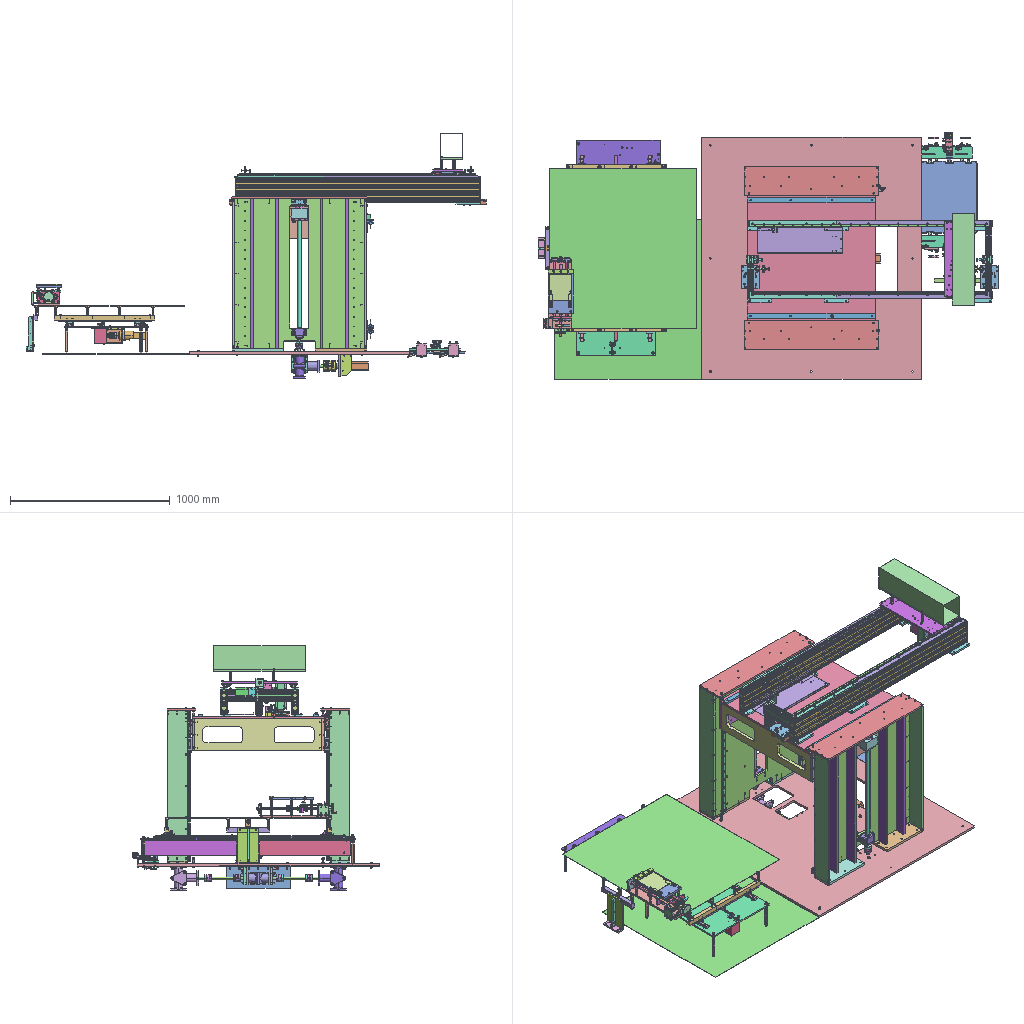Assembly | STEP file | 426 different items | 1257 placed | box 2879 x 1545 x 1531 mm
Parts list (item | name | quantity | parent item | size | volume), first 276 of 426 items:
1 | 0232_201_Base_Plate | x1 | in _0232_SA01 | 140 x 430 x 12 mm | 707820 mm3
2 | 0232_212_Work_Base | x1 | in _0232_SA01 | 155 x 275 x 14 mm | 537232 mm3
3 | 0232_213_Plate | x1 | in _0232_SA01 | 155 x 25 x 10 mm | 36548 mm3
4 | 0232_014_SLSBWRK10-100 | x6 | in _0232_SA01 | 109 x 11.5 x 10 mm | 8630 mm3
5 | 0232_Z_SCBS6-20_1 | x10 | in 0232_018_SCBS6-20 | 26 x 10 x 10 mm | 916.516 mm3
6 | 0232_Z_SCBS6-20_2 | x10 | in 0232_018_SCBS6-20 | 1.5 x 11.5 x 11.317 mm | 101.28 mm3
7 | 0232_Z_SCBS6-20_3 | x10 | in 0232_018_SCBS6-20 | 1.6 x 12.5 x 12.5 mm | 151.111 mm3
8 | 0232_301_CBM6-15 | x13 | in _0232_SA01, _0232_SA02 | 21 x 10 x 10 mm | 822.712 mm3
9 | 0232_202_Plate | x1 | in _0232_SA02 | 140 x 10 x 77 mm | 94013 mm3
10 | 0232_203_Plate | x1 | in _0232_SA02 | 140 x 10 x 77 mm | 97359 mm3
11 | 0232_204_Holder | x1 | in _0232_SA02 | 72 x 16 x 55 mm | 37017 mm3
12 | 0232_205_Plate | x1 | in _0232_SA02 | 135 x 10 x 55 mm | 54422 mm3
13 | 0232_209_Plate | x1 | in _0232_SA02 | 155 x 24 x 10 mm | 35695 mm3
14 | 0232_210_Plate | x1 | in _0232_SA02 | 20 x 170 x 6 mm | 20020 mm3
15 | 0232_211_Slide_Plate | x1 | in _0232_SA02 | 24 x 10 x 6 mm | 1162 mm3
16 | 0232_214_Bushing_Holder | x2 | in _0232_SA02 | 24 x 35 x 45 mm | 11502 mm3
17 | 0232_012_PPS12 | x1 | in _0232_SA02 | 16 x 12 x 0.5 mm | 66.945 mm3
18 | 0232_Z_CLMS5-20-B_1 | x1 | in 0232_011_CLMS5-20-B | 51.5 x 31 x 13 mm | 5282 mm3
19 | 0232_Z_CLMS5-20-B_2 | x1 | in 0232_011_CLMS5-20-B | 10 x 45.8 x 10 mm | 1925 mm3
20 | 0232_Z_UMSB6-20_1 | x2 | in 0232_010_UMSB6-20 | 5 x 20 x 20 mm | 686.512 mm3
21 | 0232_Z_UMSB6-20_2 | x2 | in 0232_010_UMSB6-20 | 5 x 15 x 15 mm | 647.79 mm3
22 | 0232_009_SETK10-26-M5-N4 | x2 | in _0232_SA02 | 41 x 10 x 10 mm | 2435 mm3
23 | 0232_008_JZB15-10 | x4 | in _0232_SA02 | 10 x 17 x 17 mm | 493.192 mm3
24 | 0232_Z_SSCSPD15_1 | x4 | in 0232_007_SSCSPD15 | 18 x 39.972 x 19.25 mm | 7194 mm3
25 | 0232_Z_SSCSPD15_2 | x4 | in 0232_007_SSCSPD15 | 10 x 10 x 22 mm | 829.902 mm3
26 | 0232_Z_SSCSPD15_3 | x4 | in 0232_007_SSCSPD15 | 10 x 10 x 22 mm | 829.902 mm3
27 | 0232_Z_SSCSPD15_4 | x4 | in 0232_007_SSCSPD15 | 18 x 39.974 x 19.251 mm | 8748 mm3
28 | 0232_Z_SSCSM15-12_1 | x4 | in 0232_006_SSCSM15-12 | 12 x 34.984 x 35 mm | 7867 mm3
29 | 0232_Z_SSCSM15-12_2 | x4 | in 0232_006_SSCSM15-12 | 8.5 x 8.5 x 21 mm | 547.959 mm3
30 | 0232_005_PSSFG15-395 | x2 | in _0232_SA02 | 395 x 15 x 15 mm | 69791 mm3
31 | 0232_Z_HBRS12_1 | x2 | in 0232_004_HBRS12 | 38 x 63 x 19 mm | 12458 mm3
32 | 0232_Z_HBRS12_2 | x2 | in 0232_004_HBRS12 | 4 x 4 x 4 mm | 41.33 mm3
33 | 0232_Z_HBRS12_3 | x2 | in 0232_004_HBRS12 | 4 x 4 x 4 mm | 41.33 mm3
34 | 0232_Z_HOKW63_1 | x1 | in 0232_003_HOKW63 | 32 x 62.998 x 62.995 mm | 57200 mm3
35 | 0232_Z_HOKW63_2 | x1 | in 0232_003_HOKW63 | 29.8 x 14 x 14 mm | 3308 mm3
36 | 0232_Z_HOKW63_3 | x1 | in 0232_003_HOKW63 | 5 x 5 x 5 mm | 80.427 mm3
37 | 0232_002_MTSFJR16 | x1 | in _0232_SA02 | 35 x 51 x 51 mm | 24502 mm3
38 | 0232_001_MTSTR16-474 | x1 | in _0232_SA02 | 474 x 16 x 16 mm | 81256 mm3
39 | 0232_Z_SCBS5-20_1 | x14 | in 0232_016_SCBS5-20 | 25 x 8.5 x 8.5 mm | 612.597 mm3
40 | 0232_Z_SCBS5-20_2 | x14 | in 0232_016_SCBS5-20 | 1.3 x 8.5 x 8.365 mm | 43.318 mm3
41 | 0232_Z_SCBS5-20_3 | x14 | in 0232_016_SCBS5-20 | 1 x 10 x 10 mm | 58.905 mm3
42 | 0232_Z_SCBS4-15_1 | x4 | in 0232_015_SCBS4-15 | 19 x 7 x 7 mm | 311.056 mm3
43 | 0232_Z_SCBS4-15_2 | x4 | in 0232_015_SCBS4-15 | 1 x 7 x 6.889 mm | 23.242 mm3
44 | 0232_Z_SCBS4-15_3 | x4 | in 0232_015_SCBS4-15 | 0.8 x 9 x 9 mm | 40.841 mm3
45 | 0232_Z_SCBS5-25_1 | x8 | in 0232_017_SCBS5-25 | 30 x 8.5 x 8.5 mm | 710.772 mm3
46 | 0232_Z_SCBS5-25_2 | x8 | in 0232_017_SCBS5-25 | 1.3 x 8.5 x 8.365 mm | 43.318 mm3
47 | 0232_Z_SCBS5-25_3 | x8 | in 0232_017_SCBS5-25 | 1 x 10 x 10 mm | 58.905 mm3
48 | 0232_Z_SCBJ2-5_1 | x2 | in 0232_019_SCBJ2-5 | 6.282 x 3.5 x 3.5 mm | 23.426 mm3
49 | 0232_Z_SCBJ2-5_2 | x2 | in 0232_019_SCBJ2-5 | 0.7 x 4 x 3.936 mm | 5.882 mm3
50 | 0232_Z_SCBJ2-5_3 | x2 | in 0232_019_SCBJ2-5 | 0.3 x 6 x 6 mm | 7.54 mm3
51 | 0232_302_CBM3-6 | x4 | in _0232_SA02 | 9 x 5.5 x 5.5 mm | 104.607 mm3
52 | 0232_303_CBM4-8 | x2 | in _0232_SA02 | 12 x 7 x 7 mm | 236.857 mm3
53 | 0232_304_SPWF4 | x2 | in _0232_SA02 | 9 x 9 x 0.8 mm | 39.276 mm3
54 | 0232_206_Plate | x1 | in _0232_SA03 | 55 x 60 x 6 mm | 18420 mm3
55 | 0232_207_Plate | x1 | in _0232_SA03 | 10 x 60 x 61 mm | 35801 mm3
56 | 0232_208_Plate | x1 | in _0232_SA03 | 30 x 60 x 6 mm | 9855 mm3
57 | 0232_013_TMEPN-2000 | x1 | in _0232_SA03 | 60 x 12 x 0.5 mm | 359.998 mm3
58 | 0232_A_Work | x1 | in Gantry loading and unloading transfer manipulator | 140 x 165 x 3 mm | 69300 mm3
59 | 0243_001_FWSSM-D7-V4-T4 | x16 | in _0243_SSA01, _0243_SA01, _0243_SSA02, _0243_SA02 | 7 x 7 x 4 mm | 102.29 mm3
60 | 0243_009_MSC5-10 | x12 | in _0243_SSA01, _0243_SA01, _0243_SSA02, _0243_SA02 | 10 x 5 x 5 mm | 181.449 mm3
61 | 0243_010_RLLUP20-50 | x10 | in _0243_SSA01, _0243_SSA02, _0243_SA04 | 20 x 73 x 20 mm | 8708 mm3
62 | 0243_Z_SCBS4-8_1 | x2 | in 0243_018_SCBS4-8 | 12 x 7 x 7 mm | 223.092 mm3
63 | 0243_Z_SCBS4-8_2 | x2 | in 0243_018_SCBS4-8 | 1 x 7 x 6.889 mm | 23.242 mm3
64 | 0243_Z_SCBS4-8_3 | x3 | in 0243_018_SCBS4-8, 0243_025_SCBZ4-8 | 0.8 x 9 x 9 mm | 40.841 mm3
65 | 0243_Z_SCBS4-10_1 | x2 | in 0243_019_SCBS4-10 | 14 x 7 x 7 mm | 248.224 mm3
66 | 0243_Z_SCBS4-10_2 | x2 | in 0243_019_SCBS4-10 | 1 x 7 x 6.889 mm | 23.242 mm3
67 | 0243_Z_SCBS4-10_3 | x2 | in 0243_019_SCBS4-10 | 0.8 x 9 x 9 mm | 40.841 mm3
68 | 0243_Z_SCBS4-16_1 | x6 | in 0243_021_SCBS4-16 | 20 x 7 x 7 mm | 323.623 mm3
69 | 0243_Z_SCBS4-16_2 | x6 | in 0243_021_SCBS4-16 | 1 x 7 x 6.889 mm | 23.242 mm3
70 | 0243_Z_SCBS4-16_3 | x6 | in 0243_021_SCBS4-16 | 0.8 x 9 x 9 mm | 40.841 mm3
71 | 0243_201_Plate | x2 | in _0243_SSA01, _0243_SSA02 | 40 x 3 x 65 mm | 7602 mm3
72 | 0243_203_Plate | x1 | in _0243_SSA01 | 8 x 73.5 x 50 mm | 28975 mm3
73 | 0243_204_Push_Plate | x2 | in _0243_SSA01, _0243_SSA02 | 30 x 2 x 50 mm | 2873 mm3
74 | 0243_218_Bar | x2 | in _0243_SSA01, _0243_SSA02 | 630 x 30 x 25 mm | 456558 mm3
75 | 0243_219_Plate | x1 | in _0243_SSA01 | 580 x 10 x 50 mm | 272354 mm3
76 | 0243_222_Dog | x1 | in _0243_SSA01 | 15 x 22 x 20 mm | 675.315 mm3
77 | socket head cap screw_iso_ISO 4762 M4 x 16 --- 16N | x5 | in _0243_SSA01, _0243_SSA02, _0243_SA02, _0243_SA04 | 20 x 7 x 7 mm | 335.506 mm3
78 | 0243_305_SCB5-18 | x5 | in _0243_SSA01, _0243_SSA02, _0243_SA03 | 23 x 8.5 x 8.5 mm | 594.23 mm3
79 | socket head cap screw_iso_ISO 4762 M5 x 40 --- 22N | x2 | in _0243_SSA01, _0243_SSA02 | 45 x 8.5 x 8.5 mm | 1026 mm3
80 | 0243_310_PWF5 | x7 | in _0243_SSA01, _0243_SSA02, _0243_SA03 | 1 x 10 x 10 mm | 56.478 mm3
81 | 0243_312_SLW5 | x7 | in _0243_SSA01, _0243_SSA02, _0243_SA03 | 1.3 x 9.2 x 9.198 mm | 58.481 mm3
82 | 0243_007_PLSBWF14-150 | x8 | in _0243_SA01, _0243_SA02 | 162 x 16.166 x 14 mm | 25375 mm3
83 | 0243_014_FPML54 | x3 | in _0243_SA01 | 26 x 19.5 x 15.5 mm | 2134 mm3
84 | 0243_015_FPCN14H-1 | x3 | in _0243_SA01 | 13 x 27 x 6 mm | 1042 mm3
85 | 0243_Z_SXR28-520_1 | x4 | in 0243_016_SXR28-520, 0243_016_SXR28-520_1 | 20 x 15.5 x 520 mm | 142241 mm3
86 | 0243_Z_SXR28-520_2 | x4 | in 0243_016_SXR28-520, 0243_016_SXR28-520_1 | 42 x 22.5 x 80 mm | 49565 mm3
87 | 0243_Z_SCBS3-5_1 | x3 | in 0243_017_SCBS3-5 | 8 x 5.5 x 5.5 mm | 92.14 mm3
88 | 0243_Z_SCBS3-5_2 | x3 | in 0243_017_SCBS3-5 | 0.7 x 5.5 x 5.413 mm | 10.455 mm3
89 | 0243_Z_SCBS3-5_3 | x3 | in 0243_017_SCBS3-5 | 0.5 x 7 x 7 mm | 15.708 mm3
90 | 0243_Z_SCBS4-12_1 | x8 | in 0243_020_SCBS4-12 | 16 x 7 x 7 mm | 273.357 mm3
91 | 0243_Z_SCBS4-12_2 | x8 | in 0243_020_SCBS4-12 | 1 x 7 x 6.889 mm | 23.242 mm3
92 | 0243_Z_SCBS4-12_3 | x8 | in 0243_020_SCBS4-12 | 0.8 x 9 x 9 mm | 40.841 mm3
93 | 0243_Z_SCBS8-25_1 | x8 | in 0243_024_SCBS8-25 | 33 x 13 x 13 mm | 2083 mm3
94 | 0243_Z_SCBS8-25_2 | x8 | in 0243_024_SCBS8-25 | 2 x 14.5 x 14.27 mm | 205.694 mm3
95 | 0243_Z_SCBS8-25_3 | x8 | in 0243_024_SCBS8-25 | 1.6 x 17 x 17 mm | 282.743 mm3
96 | 0243_202_Plate | x1 | in _0243_SA01 | 525 x 10 x 625 mm | 3182017 mm3
97 | 0243_224_Plate | x3 | in _0243_SA01 | 40 x 1.5 x 20 mm | 1142 mm3
98 | socket head cap screw_iso_ISO 4762 M3 x 8 --- 8N | x4 | in _0243_SA01 | 11 x 5.5 x 5.5 mm | 118.768 mm3
99 | socket head cap screw_iso_ISO 4762 M5 x 16 --- 16N | x4 | in _0243_SA01, _0243_SA02 | 21 x 8.5 x 8.5 mm | 554.946 mm3
100 | 0243_211_Plate | x1 | in _0243_SSA02 | 8 x 99.5 x 50 mm | 39443 mm3
101 | 0243_223_Plate | x1 | in _0243_SSA02 | 580 x 10 x 50 mm | 286525 mm3
102 | 0243_210_Plate | x1 | in _0243_SA02 | 495 x 10 x 620 mm | 2967020 mm3
103 | 0243_212_Block | x1 | in _0243_SA02 | 40 x 15 x 15 mm | 7396 mm3
104 | 0243_214_Block | x1 | in _0243_SA02 | 40 x 15 x 15 mm | 7679 mm3
105 | socket head cap screw_iso_ISO 4762 M6 x 25 --- 25N | x1 | in _0243_SA02 | 31 x 10 x 10 mm | 1098 mm3
106 | 0243_311_PWF6 | x2 | in _0243_SA02 | 1.6 x 12.5 x 12.5 mm | 144.878 mm3
107 | 0243_313_SLW6 | x2 | in _0243_SA02 | 1.5 x 12.2 x 12.197 mm | 128.674 mm3
108 | 0243_314_RCB6-65 | x1 | in _0243_SA02 | 69 x 11.547 x 10 mm | 2180 mm3
109 | 0243_315_LBNR6 | x1 | in _0243_SA02 | 5 x 11.5 x 10 mm | 332.083 mm3
110 | 0243_002_FWSSM-D15-V12-T6.2 | x2 | in _0243_SA03 | 15 x 15 x 6.2 mm | 391.034 mm3
111 | 0243_Z_B6901ZZNR_1 | x2 | in 0243_003_B6901ZZNR | 6 x 24 x 24 mm | 1839 mm3
112 | 0243_Z_B6901ZZNR_2 | x2 | in 0243_003_B6901ZZNR | 0.7 x 26.749 x 26.8 mm | 106.046 mm3
113 | 0243_004_PSFHR12-48-KFC20-G8-AG90 | x1 | in _0243_SA03 | 48 x 12 x 12 mm | 5347 mm3
114 | 0243_005_PLSBRK7-35 | x1 | in _0243_SA03 | 35 x 8.083 x 7 mm | 1328 mm3
115 | PN_0001_Z_PSCLSJ10-14_1_Default | x1 | in PN_0001_026_PSCLSJ10-14_Default | 25 x 24.977 x 12 mm | 3181 mm3
116 | PN_0001_Z_PSCLSJ10-14_2_Default | x1 | in PN_0001_026_PSCLSJ10-14_Default | 13 x 5.5 x 5.5 mm | 130.611 mm3
117 | 0243_008_B6000ZZ | x2 | in _0243_SA03 | 8 x 26 x 26 mm | 3459 mm3
118 | 0243_Z_ATPP12L050-B-P14-KC90_2 | x1 | in 0243_011_ATPP12L050-B-P14-KC90 | 45 x 31.302 x 45 mm | 20799 mm3
119 | socket set screw flat point_iso_ISO 4026 - M5 x 4-N | x2 | in 0243_011_ATPP12L050-B-P14-KC90 | 4 x 5 x 5 mm | 62.894 mm3
120 | 0243_Z_ATPP12L050-A-P12-KC90_2 | x1 | in 0243_012_ATPP12L050-A-P12-KC90 | 45 x 19.604 x 45 mm | 16570 mm3
121 | socket set screw flat point_iso_ISO 4026 - M4 x 3-N | x2 | in 0243_012_ATPP12L050-A-P12-KC90 | 3 x 4 x 4 mm | 28.895 mm3
122 | 0243_Z_MCSLC40-10-16_1 | x1 | in 0243_013_MCSLC40-10-16 | 47 x 40 x 40 mm | 40763 mm3
123 | 0243_Z_MCSLC40-10-16_2 | x1 | in 0243_013_MCSLC40-10-16 | 8.5 x 25.233 x 8.844 mm | 622.138 mm3
124 | 0243_Z_MCSLC40-10-16_3 | x1 | in 0243_013_MCSLC40-10-16 | 8.5 x 25.233 x 8.844 mm | 622.138 mm3
125 | 0243_Z_SCBS5-20_1 | x2 | in 0243_023_SCBS5-20 | 25 x 8.5 x 8.5 mm | 612.597 mm3
126 | 0243_Z_SCBS5-20_2 | x2 | in 0243_023_SCBS5-20 | 1.3 x 8.5 x 8.365 mm | 43.318 mm3
127 | 0243_Z_SCBS5-20_3 | x2 | in 0243_023_SCBS5-20 | 1 x 10 x 10 mm | 58.905 mm3
128 | 0243_101_Belt_050-L-0396A-J | x1 | in _0243_SA03 | 13.5 x 37.6 x 1267 mm | 69386 mm3
129 | 0243_102_Servo_Motor_HF-KP13G7 1_5 | x1 | in _0243_SA03 | 204.4 x 60 x 60 mm | 372734 mm3
130 | 0243_213_Plate | x2 | in _0243_SA03 | 8 x 85 x 40 mm | 23199 mm3
131 | 0243_215_Plate | x1 | in _0243_SA03 | 35 x 10 x 40 mm | 13250 mm3
132 | 0243_216_Shaft | x1 | in _0243_SA03 | 83.5 x 14 x 14 mm | 9237 mm3
133 | 0243_217_Housing | x1 | in _0243_SA03 | 25 x 87.5 x 38 mm | 70422 mm3
134 | 0243_220_Plate | x1 | in _0243_SA03 | 117 x 10 x 66 mm | 74310 mm3
135 | 0243_221_Plate | x1 | in _0243_SA03 | 10 x 97.5 x 66 mm | 38364 mm3
136 | socket head cap screw_iso_ISO 4762 M5 x 12 --- 12N | x1 | in _0243_SA03 | 17 x 8.5 x 8.5 mm | 476.406 mm3
137 | 0243_225_Cover | x1 | in _0243_SA03 | 112 x 98.5 x 68 mm | 54061 mm3
138 | 0243_316_NKJ3-8 | x1 | in _0243_SA03 | 9.961 x 5.5 x 5.5 mm | 89.104 mm3
139 | 0243_Z_SCBS4-20_1 | x1 | in 0243_022_SCBS4-20 | 24 x 7 x 7 mm | 373.888 mm3
140 | 0243_Z_SCBS4-20_2 | x1 | in 0243_022_SCBS4-20 | 1 x 7 x 6.889 mm | 23.242 mm3
141 | 0243_Z_SCBS4-20_3 | x1 | in 0243_022_SCBS4-20 | 0.8 x 9 x 9 mm | 40.841 mm3
142 | 0243_Z_SCBZ4-8_1 | x1 | in 0243_025_SCBZ4-8 | 12 x 7 x 7 mm | 217.563 mm3
143 | 0243_Z_SCBZ4-8_2 | x1 | in 0243_025_SCBZ4-8 | 1 x 7 x 7 mm | 30.412 mm3
144 | 0243_104_Sensor_EE-SPY402 | x1 | in _0243_SA04 | 7 x 20 x 26 mm | 2123 mm3
145 | 0243_105_Sensor_EE-1003 | x1 | in _0243_SA04 | 12.5 x 4.9 x 10.7 mm | 548.755 mm3
146 | 0243_106_Sensor_EE-1003A | x1 | in _0243_SA04 | 25.5 x 19 x 4.7 mm | 99.726 mm3
147 | 0243_205_Plate | x1 | in _0243_SA04 | 10 x 210 x 130 mm | 271869 mm3
148 | 0243_206_Plate | x1 | in _0243_SA04 | 50 x 10 x 130 mm | 61174 mm3
149 | 0243_207_Rib | x1 | in _0243_SA04 | 39 x 210 x 10 mm | 52975 mm3
150 | 0243_208_Plate | x1 | in _0243_SA04 | 31 x 50 x 30 mm | 4315 mm3
151 | 0243_209_Bar | x1 | in _0243_SA04 | 25 x 30 x 270 mm | 201534 mm3
152 | 0243_Work-A | x2 | in _0243_Assy, Gantry loading and unloading transfer manipulator | 919 x 2.2 x 1000 mm | 2021800 mm3
153 | 0243_226_Cover | x1 | in _0243_Assy | 1302 x 99 x 105 mm | 796517 mm3
154 | PN_0001_316_TRSS4-5_Default | x1 | in _0243_Assy | 7.372 x 9.4 x 9.4 mm | 153.282 mm3
155 | 0243_318_SCB4-6 | x1 | in _0243_Assy | 10 x 7 x 7 mm | 210.032 mm3
156 | 0243_319_PWF4 | x1 | in _0243_Assy | 0.8 x 9 x 9 mm | 40.841 mm3
157 | 0243_320_SLW4 | x1 | in _0243_Assy | 1 x 7 x 6.889 mm | 23.242 mm3
158 | 0244_201_Plate | x1 | in _0244_SA01 | 1375 x 15 x 1515 mm | 27581245 mm3
159 | 0244_216_Plate | x1 | in _0244_SA01 | 15 x 140 x 400 mm | 795604 mm3
160 | 0244_215_Rib | x2 | in _0244_SA01 | 69 x 135 x 10 mm | 86315 mm3
161 | 0244_218_Block | x2 | in _0244_SA01 | 100 x 20 x 20 mm | 34911 mm3
162 | 0244_219_Plate | x2 | in _0244_SA01 | 100 x 118 x 15 mm | 164130 mm3
163 | 0244_101_HF-KP73BG7(1-5) | x1 | in _0244_SA01 | 228 x 60 x 60 mm | 588290 mm3
164 | 0244_Z_102_ARA610LR_1 | x1 | in 0244_102_ARA610LR | 152 x 176 x 76 mm | 868653 mm3
165 | 0244_Z_102_ARA610LR_2 | x3 | in 0244_102_ARA610LR | 62 x 20 x 20 mm | 18667 mm3
166 | 0244_Z_006_SUST10-50_1 | x8 | in 0244_006_SUST10-50 | 59 x 19.63 x 17 mm | 5927 mm3
167 | 0244_Z_006_SUST10-50_2 | x8 | in 0244_006_SUST10-50 | 6 x 19.63 x 17 mm | 1142 mm3
168 | 0244_Z_007_CPSWC65-16-20_1 | x1 | in 0244_007_CPSWC65-16-20 | 77 x 65 x 65 mm | 173127 mm3
169 | 0244_Z_007_CPSWC65-16-20_2 | x8 | in 0244_007_CPSWC65-16-20 | 25.82 x 10 x 10 mm | 940.164 mm3
170 | 0244_Z_007_CPSWC65-16-20_3 | x2 | in 0244_007_CPSWC65-16-20 | 10 x 10 x 25.82 mm | 940.164 mm3
171 | 0244_Z_018_SCBS8-35_1 | x3 | in 0244_018_SCBS8-35 | 43 x 13 x 13 mm | 2585 mm3
172 | 0244_Z_018_SCBS8-35_2 | x3 | in 0244_018_SCBS8-35 | 2 x 14.5 x 14.27 mm | 205.694 mm3
173 | 0244_Z_018_SCBS8-35_3 | x3 | in 0244_018_SCBS8-35 | 1.6 x 17 x 17 mm | 282.743 mm3
174 | 0244_Z_008_MFJC44-20-20_1 | x4 | in 0244_008_MFJC44-20-20 | 14 x 44.3 x 44.3 mm | 11853 mm3
175 | 0244_Z_008_MFJC44-20-20_2 | x4 | in 0244_008_MFJC44-20-20 | 24 x 44 x 43.977 mm | 18858 mm3
176 | 0244_Z_008_MFJC44-20-20_3 | x8 | in 0244_008_MFJC44-20-20 | 8.5 x 22.82 x 8.5 mm | 582.868 mm3
177 | 0244_Z_008_MFJC44-20-20_4 | x4 | in 0244_008_MFJC44-20-20 | 24 x 43.977 x 44 mm | 18858 mm3
178 | 0244_302_SCB5-25 | x2 | in _0244_SA01 | 30 x 8.5 x 8.5 mm | 732.74 mm3
179 | 0244_309_SLW5 | x3 | in _0244_SA01 | 1.3 x 9.2 x 9.198 mm | 58.481 mm3
180 | 0244_305_SCB8-30 | x2 | in _0244_SA01 | 38 x 13 x 13 mm | 2418 mm3
181 | 0244_310_SLW8 | x8 | in _0244_SA01, _0244_SA02, _0244_SA03 | 2 x 15.4 x 15.396 mm | 260.908 mm3
182 | 0244_306_SCB8-40 | x5 | in _0244_SA01, _0244_SA02, _0244_SA03 | 48 x 13 x 13 mm | 2919 mm3
183 | 0244_311_PWF8 | x6 | in _0244_SA01, _0244_SA02, _0244_SA03 | 1.6 x 15.5 x 15.5 mm | 213.239 mm3
184 | 0244_308_SLBNR8 | x3 | in _0244_SA01, _0244_SA02, _0244_SA03 | 13 x 6.5 x 15.011 mm | 690.678 mm3
185 | 0244_312_SCB5-15 | x1 | in _0244_SA01 | 20 x 8.5 x 8.5 mm | 536.391 mm3
186 | 0244_202_Plate | x2 | in _0244_SA02, _0244_SA03 | 810 x 940 x 15 mm | 9838794 mm3
187 | 0244_203_Spacer | x2 | in _0244_SA02, _0244_SA03 | 95 x 42 x 9 mm | 32489 mm3
188 | 0244_204_Block | x2 | in _0244_SA02, _0244_SA03 | 100 x 60 x 130 mm | 602094 mm3
189 | 0244_205_Spacer | x2 | in _0244_SA02, _0244_SA03 | 95 x 26 x 9 mm | 20519 mm3
190 | 0244_206_Rib | x8 | in _0244_SA02, _0244_SA03 | 15 x 940 x 69 mm | 970770 mm3
191 | 0244_209_Plate | x4 | in _0244_SA02, _0244_SA03 | 15 x 940 x 125 mm | 1754241 mm3
192 | 0244_217_Plate | x2 | in _0244_SA02, _0244_SA03 | 840 x 12 x 180 mm | 1806542 mm3
193 | 0244_220_Blacket | x3 | in _0244_SA02 | 35 x 25 x 20 mm | 2572 mm3
194 | 0244_013_SENAF3-120 | x2 | in _0244_SA02 | 120 x 9 x 6 mm | 3722 mm3
195 | 0244_Z_001_BSST2510-1195_2 | x2 | in 0244_001_BSST2510-1195 | 92 x 96 x 60 mm | 221226 mm3
196 | 0244_Z_001_BSST2510-1195_1 | x2 | in 0244_001_BSST2510-1195 | 895 x 25 x 25 mm | 414687 mm3
197 | 0244_Z_001_BSST2510-1195_3 | x2 | in 0244_001_BSST2510-1195 | 20 x 25 x 25 mm | 3534 mm3
198 | 0244_Z_002_BSW20_1 | x2 | in 0244_002_BSW20 | 52 x 58 x 95 mm | 184374 mm3
199 | 0244_Z_002_BSW20_2 | x2 | in 0244_002_BSW20 | 11 x 25 x 25 mm | 1944 mm3
200 | 0244_Z_002_BSW20_3 | x2 | in 0244_002_BSW20 | 13 x 35 x 35 mm | 6873 mm3
201 | 0244_Z_003_BUN20_1 | x2 | in 0244_003_BUN20 | 26 x 58 x 95 mm | 83295 mm3
202 | 0244_Z_003_BUN20_2 | x2 | in 0244_003_BUN20 | 1.75 x 47.073 x 49.5 mm | 834.57 mm3
203 | 0244_Z_003_BUN20_3 | x2 | in 0244_003_BUN20 | 1.2 x 25.6 x 23.05 mm | 179.471 mm3
204 | 0244_Z_004_SX2W33-1240_1 | x4 | in 0244_004_SX2W33-1240 | 23 x 18 x 940 mm | 339429 mm3
205 | 0244_Z_004_SX2W33-1240_2 | x4 | in 0244_004_SX2W33-1240 | 73 x 26.5 x 96 mm | 100678 mm3
206 | 0244_Z_004_SX2W33-1240_3 | x4 | in 0244_004_SX2W33-1240 | 73 x 26.5 x 96 mm | 100678 mm3
207 | 0244_005_PSSFG20-160 | x2 | in _0244_SA02, _0244_SA03 | 160 x 20 x 20 mm | 50205 mm3
208 | 0244_Z_009_MFJC44-15-20_1 | x2 | in 0244_009_MFJC44-15-20 | 14 x 44.3 x 44.3 mm | 11853 mm3
209 | 0244_Z_009_MFJC44-15-20_2 | x2 | in 0244_009_MFJC44-15-20 | 24 x 44 x 43.977 mm | 20844 mm3
210 | 0244_Z_009_MFJC44-15-20_3 | x4 | in 0244_009_MFJC44-15-20 | 8.5 x 22.82 x 8.5 mm | 582.868 mm3
211 | 0244_Z_009_MFJC44-15-20_4 | x2 | in 0244_009_MFJC44-15-20 | 24 x 43.977 x 44 mm | 18858 mm3
212 | 0244_010_MSC6-15 | x2 | in _0244_SA02, _0244_SA03 | 15 x 6 x 6 mm | 396.61 mm3
213 | 0244_011_FPML54 | x3 | in _0244_SA02 | 26 x 19.5 x 15.5 mm | 2111 mm3
214 | 0244_012_FPCN14H | x3 | in _0244_SA02 | 13 x 45 x 6 mm | 1495 mm3
215 | 0244_Z_014_SCBS3-6_1 | x1 | in 0244_014_SCBS3-6 | 9 x 5.5 x 5.5 mm | 99.208 mm3
216 | 0244_Z_014_SCBS3-6_2 | x1 | in 0244_014_SCBS3-6 | 0.7 x 5.5 x 5.413 mm | 10.455 mm3
217 | 0244_Z_014_SCBS3-6_3 | x1 | in 0244_014_SCBS3-6 | 0.5 x 7 x 7 mm | 15.708 mm3
218 | 0244_016_SCBS6-30 | x2 | in _0244_SA02, _0244_SA03 | 36 x 12.5 x 12.5 mm | 1452 mm3
219 | 0244_Z_017_SCBS8-30_1 | x3 | in 0244_017_SCBS8-30 | 38 x 13 x 13 mm | 2334 mm3
220 | 0244_Z_017_SCBS8-30_2 | x3 | in 0244_017_SCBS8-30 | 2 x 14.5 x 14.27 mm | 205.694 mm3
221 | 0244_Z_017_SCBS8-30_3 | x3 | in 0244_017_SCBS8-30 | 1.6 x 17 x 17 mm | 282.743 mm3
222 | 0244_Z_019_SCBZ6-25_1 | x4 | in 0244_019_SCBZ6-25 | 31 x 10 x 10 mm | 1045 mm3
223 | 0244_Z_019_SCBZ6-25_2 | x4 | in 0244_019_SCBZ6-25 | 1.5 x 10 x 10 mm | 91.887 mm3
224 | 0244_Z_104_ARA610SN_1 | x1 | in 0244_104_ARA610SN | 152 x 176 x 76 mm | 868653 mm3
225 | 0244_Z_104_ARA610SN_2 | x2 | in 0244_104_ARA610SN | 62 x 20 x 20 mm | 18667 mm3
226 | 0244_301_SCB3-6 | x1 | in _0244_SA02 | 9 x 5.5 x 5.5 mm | 103.858 mm3
227 | 0244_303_SCB6-20 | x2 | in _0244_SA02, _0244_SA03 | 26 x 10 x 10 mm | 958.655 mm3
228 | 0244_304_SCB6-25 | x8 | in _0244_SA02, _0244_SA03, _0244_SA04 | 31 x 10 x 10 mm | 1100 mm3
229 | 0244_307_SCB10-50 | x4 | in _0244_SA02, _0244_SA03 | 60 x 16 x 16 mm | 5603 mm3
230 | 0244_208_Plate | x2 | in _0244_SA02, _0244_SA03 | 320 x 16 x 125 mm | 627294 mm3
231 | 0244_223_Plate | x2 | in _0244_SA02, _0244_SA03 | 320 x 16 x 125 mm | 627294 mm3
232 | 0244_Z_103_ARA610SF_1 | x1 | in 0244_103_ARA610SF | 152 x 176 x 76 mm | 868653 mm3
233 | 0244_Z_103_ARA610SF_2 | x2 | in 0244_103_ARA610SF | 62 x 20 x 20 mm | 18667 mm3
234 | 0244_207_Plate | x1 | in _0244_SA04 | 800 x 15 x 826 mm | 9900374 mm3
235 | 0244_210_Plate | x2 | in _0244_SA04 | 800 x 15 x 30 mm | 356183 mm3
236 | 0244_211_Plate | x4 | in _0244_SA04 | 20 x 200 x 796 mm | 2203908 mm3
237 | 0244_212_Plate | x1 | in _0244_SA04 | 800 x 200 x 15 mm | 2353500 mm3
238 | 0244_221_Dog | x1 | in _0244_SA04 | 46 x 30 x 32 mm | 2278 mm3
239 | 0244_222_Plate | x1 | in _0244_SA04 | 800 x 200 x 15 mm | 2359509 mm3
240 | 0244_Z_015_SCBS4-12_1 | x1 | in 0244_015_SCBS4-12 | 16 x 7 x 7 mm | 273.357 mm3
241 | 0244_Z_015_SCBS4-12_2 | x1 | in 0244_015_SCBS4-12 | 1 x 7 x 6.889 mm | 23.242 mm3
242 | 0244_Z_015_SCBS4-12_3 | x1 | in 0244_015_SCBS4-12 | 0.8 x 9 x 9 mm | 40.841 mm3
243 | 0245_208_Plate | x6 | in _0245_SA01 | 65 x 12 x 150 mm | 114653 mm3
244 | 0245_022_HFS8-40160-1530-LCH-RCH | x2 | in _0245_SA01 | 40 x 160 x 1530 mm | 3125718 mm3
245 | 0245_023_HFS8-4080-405-TPW | x1 | in _0245_SA01 | 40 x 80 x 405 mm | 451143 mm3
246 | 0245_015_HFS8-4080-225-LTP | x1 | in _0245_SA01 | 40 x 80 x 225 mm | 250637 mm3
247 | 0245_Z_016_HCJ8_1 | x2 | in 0245_016_HCJ8 | 24 x 18 x 12 mm | 710.453 mm3
248 | 0245_Z_016_HCJ8_2 | x2 | in 0245_016_HCJ8 | 18 x 18 x 33.9 mm | 3765 mm3
249 | 0245_017_HFC8-4080-S | x9 | in _0245_SA01 | 80 x 40 x 11 mm | 6318 mm3
250 | 0245_025_HFSF5-4040-82-LTP | x1 | in _0245_SA01 | 40 x 40 x 82 mm | 42687 mm3
251 | 0245_211_Plate | x1 | in _0245_SA01 | 40 x 10 x 70 mm | 25290 mm3
252 | 0245_304_SCB5-15 | x2 | in _0245_SA01, _0245_SA02 | 20 x 8.5 x 8.5 mm | 536.391 mm3
253 | 0245_Z_036_SCBS6-20_1 | x1 | in 0245_036_SCBS6-20 | 26 x 10 x 10 mm | 916.516 mm3
254 | 0245_Z_036_SCBS6-20_2 | x1 | in 0245_036_SCBS6-20 | 1.5 x 11.5 x 11.317 mm | 101.28 mm3
255 | 0245_Z_036_SCBS6-20_3 | x1 | in 0245_036_SCBS6-20 | 1.6 x 12.5 x 12.5 mm | 151.111 mm3
256 | 0245_309_SCB6-15 | x1 | in _0245_SA01 | 21 x 10 x 10 mm | 817.284 mm3
257 | 0245_019_HNTFSN8-6 | x1 | in _0245_SA01 | 8.9 x 17 x 14.908 mm | 961.616 mm3
258 | 0245_Z_037_SCBS6-25_1 | x2 | in 0245_037_SCBS6-25 | 31 x 10 x 10 mm | 1058 mm3
259 | 0245_Z_037_SCBS6-25_2 | x2 | in 0245_037_SCBS6-25 | 1.5 x 11.5 x 11.317 mm | 101.28 mm3
260 | 0245_Z_037_SCBS6-25_3 | x2 | in 0245_037_SCBS6-25 | 1.6 x 12.5 x 12.5 mm | 151.111 mm3
261 | 0245_203_Blacket | x3 | in _0245_SA01 | 32 x 20 x 30 mm | 2157 mm3
262 | 0245_Z_040_SCBS5-15_1 | x4 | in 0245_040_SCBS5-15 | 20 x 8.5 x 8.5 mm | 514.422 mm3
263 | 0245_Z_040_SCBS5-15_2 | x4 | in 0245_040_SCBS5-15 | 1.3 x 8.5 x 8.365 mm | 43.318 mm3
264 | 0245_Z_040_SCBS5-15_3 | x4 | in 0245_040_SCBS5-15 | 1 x 10 x 10 mm | 58.905 mm3
265 | 0245_012_HNTFSN8-5 | x9 | in _0245_SA01, _0245_SA02 | 8.9 x 17 x 14.908 mm | 1013 mm3
266 | 0245_217_Cable | x1 | in _0245_SA01 | 165 x 40 x 530 mm | 227644 mm3
267 | 0245_212_Blacket | x1 | in _0245_SA01 | 40 x 40 x 40 mm | 8827 mm3
268 | 0245_Z_030_SCBS4-10_1 | x2 | in 0245_030_SCBS4-10 | 14 x 7 x 7 mm | 247.861 mm3
269 | 0245_Z_030_SCBS4-10_2 | x2 | in 0245_030_SCBS4-10 | 1 x 7 x 6.889 mm | 23.242 mm3
270 | 0245_Z_030_SCBS4-10_3 | x2 | in 0245_030_SCBS4-10 | 0.8 x 9 x 9 mm | 40.841 mm3
271 | 0245_026_HNTFSN5-4 | x1 | in _0245_SA01 | 5 x 10 x 8.891 mm | 178.899 mm3
272 | 0245_204_Blacket | x2 | in _0245_SA01 | 50 x 65 x 65 mm | 36528 mm3
273 | 0245_014_HNTFSN8-8 | x1 | in _0245_SA01 | 8.9 x 17 x 14.908 mm | 816.432 mm3
274 | 0245_Z_038_SCBS8-20_1 | x1 | in 0245_038_SCBS8-20 | 28 x 13 x 13 mm | 1831 mm3
275 | 0245_Z_038_SCBS8-20_2 | x1 | in 0245_038_SCBS8-20 | 2 x 14.5 x 14.27 mm | 205.694 mm3
276 | 0245_Z_038_SCBS8-20_3 | x1 | in 0245_038_SCBS8-20 | 1.6 x 17 x 17 mm | 282.743 mm3
Placements (level | parent | child | x y z in mm | rotation matrix by rows), first 197 of 1489 lines:
1 | Gantry loading and unloading transfer manipulator | _0232_SA01 | 20.588 -201.056 -0.0 | 1 0 0 0 1 0 0 0 1
2 | _0232_SA01 | 0232_201_Base_Plate | -0.0 -0.0 -0.0 | 1 0 0 0 1 0 0 0 1
2 | _0232_SA01 | 0232_212_Work_Base | 7.5 92.5 112.0 | 1 0 0 0 1 0 0 0 1
2 | _0232_SA01 | 0232_213_Plate | -70.0 342.5 126.0 | 1 0 0 0 1 0 0 0 1
2 | _0232_SA01 | 0232_014_SLSBWRK10-100 | -132.5 355.0 12.0 | 0 0 -1 0 1 0 1 0 0
2 | _0232_SA01 | 0232_014_SLSBWRK10-100 | -7.5 355.0 12.0 | 0 0 -1 0 1 0 1 0 0
2 | _0232_SA01 | 0232_014_SLSBWRK10-100 | -7.5 230.0 12.0 | 0 0 -1 0 1 0 1 0 0
2 | _0232_SA01 | 0232_014_SLSBWRK10-100 | -132.5 230.0 12.0 | 0 0 -1 0 1 0 1 0 0
2 | _0232_SA01 | 0232_014_SLSBWRK10-100 | -92.5 105.0 12.0 | 0 0 -1 0 1 0 1 0 0
2 | _0232_SA01 | 0232_014_SLSBWRK10-100 | -7.5 105.0 12.0 | 0 0 -1 0 1 0 1 0 0
2 | _0232_SA01 | 0232_018_SCBS6-20 | -10.0 65.0 6.4 | 0 0 -1 0 1 0 1 0 0
3 | 0232_018_SCBS6-20 | 0232_Z_SCBS6-20_1 | -0.0 -0.0 -0.0 | 1 0 0 0 1 0 0 0 1
3 | 0232_018_SCBS6-20 | 0232_Z_SCBS6-20_2 | -0.0 -0.0 -0.0 | 1 0 0 0 1 0 0 0 1
3 | 0232_018_SCBS6-20 | 0232_Z_SCBS6-20_3 | -0.0 -0.0 -0.0 | 1 0 0 0 1 0 0 0 1
2 | _0232_SA01 | 0232_018_SCBS6-20 | -10.0 420.0 6.4 | 0 0 -1 0 1 0 1 0 0
3 | 0232_018_SCBS6-20 | 0232_Z_SCBS6-20_1 | -0.0 -0.0 -0.0 | 1 0 0 0 1 0 0 0 1
3 | 0232_018_SCBS6-20 | 0232_Z_SCBS6-20_2 | -0.0 -0.0 -0.0 | 1 0 0 0 1 0 0 0 1
3 | 0232_018_SCBS6-20 | 0232_Z_SCBS6-20_3 | -0.0 -0.0 -0.0 | 1 0 0 0 1 0 0 0 1
2 | _0232_SA01 | 0232_018_SCBS6-20 | -130.0 65.0 6.4 | 0 0 -1 0 1 0 1 0 0
3 | 0232_018_SCBS6-20 | 0232_Z_SCBS6-20_1 | -0.0 -0.0 -0.0 | 1 0 0 0 1 0 0 0 1
3 | 0232_018_SCBS6-20 | 0232_Z_SCBS6-20_2 | -0.0 -0.0 -0.0 | 1 0 0 0 1 0 0 0 1
3 | 0232_018_SCBS6-20 | 0232_Z_SCBS6-20_3 | -0.0 -0.0 -0.0 | 1 0 0 0 1 0 0 0 1
2 | _0232_SA01 | 0232_018_SCBS6-20 | -90.0 65.0 6.4 | 0 0 -1 0 1 0 1 0 0
3 | 0232_018_SCBS6-20 | 0232_Z_SCBS6-20_1 | -0.0 -0.0 -0.0 | 1 0 0 0 1 0 0 0 1
3 | 0232_018_SCBS6-20 | 0232_Z_SCBS6-20_2 | -0.0 -0.0 -0.0 | 1 0 0 0 1 0 0 0 1
3 | 0232_018_SCBS6-20 | 0232_Z_SCBS6-20_3 | -0.0 -0.0 -0.0 | 1 0 0 0 1 0 0 0 1
2 | _0232_SA01 | 0232_018_SCBS6-20 | -50.0 420.0 6.4 | 0 0 -1 0 1 0 1 0 0
3 | 0232_018_SCBS6-20 | 0232_Z_SCBS6-20_1 | -0.0 -0.0 -0.0 | 1 0 0 0 1 0 0 0 1
3 | 0232_018_SCBS6-20 | 0232_Z_SCBS6-20_2 | -0.0 -0.0 -0.0 | 1 0 0 0 1 0 0 0 1
3 | 0232_018_SCBS6-20 | 0232_Z_SCBS6-20_3 | -0.0 -0.0 -0.0 | 1 0 0 0 1 0 0 0 1
2 | _0232_SA01 | 0232_018_SCBS6-20 | -90.0 420.0 6.4 | 0 0 -1 0 1 0 1 0 0
3 | 0232_018_SCBS6-20 | 0232_Z_SCBS6-20_1 | -0.0 -0.0 -0.0 | 1 0 0 0 1 0 0 0 1
3 | 0232_018_SCBS6-20 | 0232_Z_SCBS6-20_2 | -0.0 -0.0 -0.0 | 1 0 0 0 1 0 0 0 1
3 | 0232_018_SCBS6-20 | 0232_Z_SCBS6-20_3 | -0.0 -0.0 -0.0 | 1 0 0 0 1 0 0 0 1
2 | _0232_SA01 | 0232_018_SCBS6-20 | -50.0 65.0 6.4 | 0 0 -1 0 1 0 1 0 0
3 | 0232_018_SCBS6-20 | 0232_Z_SCBS6-20_1 | -0.0 -0.0 -0.0 | 1 0 0 0 1 0 0 0 1
3 | 0232_018_SCBS6-20 | 0232_Z_SCBS6-20_2 | -0.0 -0.0 -0.0 | 1 0 0 0 1 0 0 0 1
3 | 0232_018_SCBS6-20 | 0232_Z_SCBS6-20_3 | -0.0 -0.0 -0.0 | 1 0 0 0 1 0 0 0 1
2 | _0232_SA01 | 0232_018_SCBS6-20 | -130.0 420.0 6.4 | 0 0 -1 0 1 0 1 0 0
3 | 0232_018_SCBS6-20 | 0232_Z_SCBS6-20_1 | -0.0 -0.0 -0.0 | 1 0 0 0 1 0 0 0 1
3 | 0232_018_SCBS6-20 | 0232_Z_SCBS6-20_2 | -0.0 -0.0 -0.0 | 1 0 0 0 1 0 0 0 1
3 | 0232_018_SCBS6-20 | 0232_Z_SCBS6-20_3 | -0.0 -0.0 -0.0 | 1 0 0 0 1 0 0 0 1
2 | _0232_SA01 | 0232_301_CBM6-15 | -7.5 105.0 119.5 | 0 0 1 0 1 0 -1 0 0
2 | _0232_SA01 | 0232_301_CBM6-15 | -25.0 355.0 129.5 | 0 0 1 0 1 0 -1 0 0
2 | _0232_SA01 | 0232_301_CBM6-15 | -132.5 355.0 119.5 | 0 0 1 0 1 0 -1 0 0
2 | _0232_SA01 | 0232_301_CBM6-15 | -115.0 355.0 129.5 | 0 0 1 0 1 0 -1 0 0
2 | _0232_SA01 | 0232_301_CBM6-15 | -70.0 355.0 129.5 | 0 0 1 0 1 0 -1 0 0
2 | _0232_SA01 | 0232_301_CBM6-15 | -92.5 105.0 119.5 | 0 0 1 0 1 0 -1 0 0
2 | _0232_SA01 | 0232_301_CBM6-15 | -7.5 230.0 119.5 | 0 0 1 0 1 0 -1 0 0
2 | _0232_SA01 | 0232_301_CBM6-15 | -7.5 355.0 119.5 | 0 0 1 0 1 0 -1 0 0
2 | _0232_SA01 | 0232_301_CBM6-15 | -132.5 230.0 119.5 | 0 0 1 0 1 0 -1 0 0
1 | Gantry loading and unloading transfer manipulator | _0232_SA02 | 20.588 -141.056 12.0 | 1 0 0 0 1 0 0 0 1
2 | _0232_SA02 | 0232_202_Plate | -0.0 -0.0 -0.0 | 1 0 0 0 1 0 0 0 1
2 | _0232_SA02 | 0232_203_Plate | -70.0 355.0 -0.0 | 1 0 0 0 1 0 0 0 1
2 | _0232_SA02 | 0232_204_Holder | -34.0 -51.0 0.0 | 1 0 0 0 1 0 0 0 1
2 | _0232_SA02 | 0232_205_Plate | -10.0 95.0 74.0 | 1 0 0 0 1 0 0 0 1
2 | _0232_SA02 | 0232_209_Plate | 6.0 81.0 74.0 | 1 0 0 0 1 0 0 0 1
2 | _0232_SA02 | 0232_210_Plate | -124.0 105.0 67.0 | 1 0 0 0 1 0 0 0 1
2 | _0232_SA02 | 0232_211_Slide_Plate | -120.0 -0.0 61.0 | 1 0 0 0 1 0 0 0 1
2 | _0232_SA02 | 0232_214_Bushing_Holder | -110.0 105.0 45.0 | 1 0 0 0 1 0 0 0 1
2 | _0232_SA02 | 0232_214_Bushing_Holder | -30.0 105.0 45.0 | 1 0 0 0 1 0 0 0 1
2 | _0232_SA02 | 0232_012_PPS12 | -132.0 -55.0 73.0 | 0 1 0 -1 0 0 0 0 1
2 | _0232_SA02 | 0232_011_CLMS5-20-B | -58.0 -43.0 55.0 | 1 0 0 0 0 -1 0 1 0
3 | 0232_011_CLMS5-20-B | 0232_Z_CLMS5-20-B_1 | -0.0 -0.0 -0.0 | 1 0 0 0 1 0 0 0 1
3 | 0232_011_CLMS5-20-B | 0232_Z_CLMS5-20-B_2 | -0.0 -0.0 -0.0 | 1 0 0 0 1 0 0 0 1
2 | _0232_SA02 | 0232_010_UMSB6-20 | -11.5 88.0 114.5 | 0 -0.6715 -0.741 0 0.741 -0.6715 1 0 0
3 | 0232_010_UMSB6-20 | 0232_Z_UMSB6-20_1 | -0.0 -0.0 -0.0 | 1 0 0 0 1 0 0 0 1
3 | 0232_010_UMSB6-20 | 0232_Z_UMSB6-20_2 | -0.0 -0.0 -0.0 | 1 0 0 0 1 0 0 0 1
2 | _0232_SA02 | 0232_010_UMSB6-20 | -131.5 88.0 114.5 | 0 0 -1 0 1 0 1 0 0
3 | 0232_010_UMSB6-20 | 0232_Z_UMSB6-20_1 | -0.0 -0.0 -0.0 | 1 0 0 0 1 0 0 0 1
3 | 0232_010_UMSB6-20 | 0232_Z_UMSB6-20_2 | -0.0 -0.0 -0.0 | 1 0 0 0 1 0 0 0 1
2 | _0232_SA02 | 0232_009_SETK10-26-M5-N4 | -131.5 88.0 86.0 | 0 0 -1 0 1 0 1 0 0
2 | _0232_SA02 | 0232_009_SETK10-26-M5-N4 | -11.5 88.0 86.0 | 0 0 -1 0 1 0 1 0 0
2 | _0232_SA02 | 0232_008_JZB15-10 | -30.0 130.0 45.0 | 0 0.3371 0.9415 -1 0 0 0 -0.9415 0.3371
2 | _0232_SA02 | 0232_008_JZB15-10 | -110.0 130.0 45.0 | 0 0.4234 0.906 -1 0 0 0 -0.906 0.4234
2 | _0232_SA02 | 0232_008_JZB15-10 | -110.0 95.0 45.0 | 0 -1 0 1 0 0 0 0 1
2 | _0232_SA02 | 0232_008_JZB15-10 | -30.0 95.0 45.0 | 0 -1 0 1 0 0 0 0 1
2 | _0232_SA02 | 0232_007_SSCSPD15 | -110.0 74.5 45.0 | 0 1 0 -1 0 0 0 0 1
3 | 0232_007_SSCSPD15 | 0232_Z_SSCSPD15_1 | -0.0 -0.0 -0.0 | 1 0 0 0 1 0 0 0 1
3 | 0232_007_SSCSPD15 | 0232_Z_SSCSPD15_2 | -0.0 -0.0 -0.0 | 1 0 0 0 1 0 0 0 1
3 | 0232_007_SSCSPD15 | 0232_Z_SSCSPD15_3 | -0.0 -0.0 -0.0 | 1 0 0 0 1 0 0 0 1
3 | 0232_007_SSCSPD15 | 0232_Z_SSCSPD15_4 | -0.0 -0.0 -0.0 | 1 0 0 0 1 0 0 0 1
2 | _0232_SA02 | 0232_007_SSCSPD15 | -110.0 191.5 45.0 | 0 1 0 -1 0 0 0 0 1
3 | 0232_007_SSCSPD15 | 0232_Z_SSCSPD15_1 | -0.0 -0.0 -0.0 | 1 0 0 0 1 0 0 0 1
3 | 0232_007_SSCSPD15 | 0232_Z_SSCSPD15_2 | -0.0 -0.0 -0.0 | 1 0 0 0 1 0 0 0 1
3 | 0232_007_SSCSPD15 | 0232_Z_SSCSPD15_3 | -0.0 -0.0 -0.0 | 1 0 0 0 1 0 0 0 1
3 | 0232_007_SSCSPD15 | 0232_Z_SSCSPD15_4 | -0.0 -0.0 -0.0 | 1 0 0 0 1 0 0 0 1
2 | _0232_SA02 | 0232_007_SSCSPD15 | -30.0 74.5 45.0 | 0 1 0 -1 0 0 0 0 1
3 | 0232_007_SSCSPD15 | 0232_Z_SSCSPD15_1 | -0.0 -0.0 -0.0 | 1 0 0 0 1 0 0 0 1
3 | 0232_007_SSCSPD15 | 0232_Z_SSCSPD15_2 | -0.0 -0.0 -0.0 | 1 0 0 0 1 0 0 0 1
3 | 0232_007_SSCSPD15 | 0232_Z_SSCSPD15_3 | -0.0 -0.0 -0.0 | 1 0 0 0 1 0 0 0 1
3 | 0232_007_SSCSPD15 | 0232_Z_SSCSPD15_4 | -0.0 -0.0 -0.0 | 1 0 0 0 1 0 0 0 1
2 | _0232_SA02 | 0232_007_SSCSPD15 | -30.0 191.5 45.0 | 0 1 0 -1 0 0 0 0 1
3 | 0232_007_SSCSPD15 | 0232_Z_SSCSPD15_1 | -0.0 -0.0 -0.0 | 1 0 0 0 1 0 0 0 1
3 | 0232_007_SSCSPD15 | 0232_Z_SSCSPD15_2 | -0.0 -0.0 -0.0 | 1 0 0 0 1 0 0 0 1
3 | 0232_007_SSCSPD15 | 0232_Z_SSCSPD15_3 | -0.0 -0.0 -0.0 | 1 0 0 0 1 0 0 0 1
3 | 0232_007_SSCSPD15 | 0232_Z_SSCSPD15_4 | -0.0 -0.0 -0.0 | 1 0 0 0 1 0 0 0 1
2 | _0232_SA02 | 0232_006_SSCSM15-12 | -110.0 -6.0 45.0 | 0 0 -1 -1 0 0 0 1 0
3 | 0232_006_SSCSM15-12 | 0232_Z_SSCSM15-12_1 | -0.0 -0.0 -0.0 | 1 0 0 0 1 0 0 0 1
3 | 0232_006_SSCSM15-12 | 0232_Z_SSCSM15-12_2 | -0.0 -0.0 -0.0 | 1 0 0 0 1 0 0 0 1
2 | _0232_SA02 | 0232_006_SSCSM15-12 | -110.0 371.0 45.0 | 0 0 -1 -1 0 0 0 1 -0
3 | 0232_006_SSCSM15-12 | 0232_Z_SSCSM15-12_1 | -0.0 -0.0 -0.0 | 1 0 0 0 1 0 0 0 1
3 | 0232_006_SSCSM15-12 | 0232_Z_SSCSM15-12_2 | -0.0 -0.0 -0.0 | 1 0 0 0 1 0 0 0 1
2 | _0232_SA02 | 0232_006_SSCSM15-12 | -30.0 371.0 45.0 | 0 0 -1 -1 0 0 0 1 -0
3 | 0232_006_SSCSM15-12 | 0232_Z_SSCSM15-12_1 | -0.0 -0.0 -0.0 | 1 0 0 0 1 0 0 0 1
3 | 0232_006_SSCSM15-12 | 0232_Z_SSCSM15-12_2 | -0.0 -0.0 -0.0 | 1 0 0 0 1 0 0 0 1
2 | _0232_SA02 | 0232_006_SSCSM15-12 | -30.0 -6.0 45.0 | 0 0 -1 -1 0 0 0 1 -0
3 | 0232_006_SSCSM15-12 | 0232_Z_SSCSM15-12_1 | -0.0 -0.0 -0.0 | 1 0 0 0 1 0 0 0 1
3 | 0232_006_SSCSM15-12 | 0232_Z_SSCSM15-12_2 | -0.0 -0.0 -0.0 | 1 0 0 0 1 0 0 0 1
2 | _0232_SA02 | 0232_005_PSSFG15-395 | -30.0 -15.0 45.0 | 0 0.8573 -0.5149 1 0 0 0 -0.5149 -0.8573
2 | _0232_SA02 | 0232_005_PSSFG15-395 | -110.0 -15.0 45.0 | 0 0.207 0.9783 1 0 0 0 0.9783 -0.207
2 | _0232_SA02 | 0232_004_HBRS12 | -70.0 374.5 45.0 | -1 0 0 0 0 1 0 1 0
3 | 0232_004_HBRS12 | 0232_Z_HBRS12_1 | -0.0 -0.0 -0.0 | 1 0 0 0 1 0 0 0 1
3 | 0232_004_HBRS12 | 0232_Z_HBRS12_2 | -0.0 -0.0 -0.0 | 1 0 0 0 1 0 0 0 1
3 | 0232_004_HBRS12 | 0232_Z_HBRS12_3 | -0.0 -0.0 -0.0 | 1 0 0 0 1 0 0 0 1
2 | _0232_SA02 | 0232_004_HBRS12 | -70.0 -9.5 45.0 | 1 0 0 0 0 -1 0 1 0
3 | 0232_004_HBRS12 | 0232_Z_HBRS12_1 | -0.0 -0.0 -0.0 | 1 0 0 0 1 0 0 0 1
3 | 0232_004_HBRS12 | 0232_Z_HBRS12_2 | -0.0 -0.0 -0.0 | 1 0 0 0 1 0 0 0 1
3 | 0232_004_HBRS12 | 0232_Z_HBRS12_3 | -0.0 -0.0 -0.0 | 1 0 0 0 1 0 0 0 1
2 | _0232_SA02 | 0232_003_HOKW63 | -70.0 -61.0 45.0 | 0 0 1 1 0 0 0 1 0
3 | 0232_003_HOKW63 | 0232_Z_HOKW63_1 | -0.0 -0.0 -0.0 | 1 0 0 0 1 0 0 0 1
3 | 0232_003_HOKW63 | 0232_Z_HOKW63_2 | -0.0 -0.0 -0.0 | 1 0 0 0 1 0 0 0 1
3 | 0232_003_HOKW63 | 0232_Z_HOKW63_3 | -0.0 -0.0 -0.0 | 1 0 0 0 1 0 0 0 1
2 | _0232_SA02 | 0232_002_MTSFJR16 | -70.0 111.0 45.0 | 0 1 0 -1 0 0 0 0 1
2 | _0232_SA02 | 0232_001_MTSTR16-474 | -70.0 -83.0 45.0 | 0 0 1 1 0 0 0 1 0
2 | _0232_SA02 | 0232_016_SCBS5-20 | -117.5 100.0 86.3 | 0 0 1 0 1 0 -1 0 0
3 | 0232_016_SCBS5-20 | 0232_Z_SCBS5-20_1 | -0.0 -0.0 -0.0 | 1 0 0 0 1 0 0 0 1
3 | 0232_016_SCBS5-20 | 0232_Z_SCBS5-20_2 | -0.0 -0.0 -0.0 | 1 0 0 0 1 0 0 0 1
3 | 0232_016_SCBS5-20 | 0232_Z_SCBS5-20_3 | -0.0 -0.0 -0.0 | 1 0 0 0 1 0 0 0 1
2 | _0232_SA02 | 0232_016_SCBS5-20 | -92.5 100.0 86.3 | 0 0 1 0 1 0 -1 0 0
3 | 0232_016_SCBS5-20 | 0232_Z_SCBS5-20_1 | -0.0 -0.0 -0.0 | 1 0 0 0 1 0 0 0 1
3 | 0232_016_SCBS5-20 | 0232_Z_SCBS5-20_2 | -0.0 -0.0 -0.0 | 1 0 0 0 1 0 0 0 1
3 | 0232_016_SCBS5-20 | 0232_Z_SCBS5-20_3 | -0.0 -0.0 -0.0 | 1 0 0 0 1 0 0 0 1
2 | _0232_SA02 | 0232_016_SCBS5-20 | -47.5 100.0 86.3 | 0 0 1 0 1 0 -1 0 0
3 | 0232_016_SCBS5-20 | 0232_Z_SCBS5-20_1 | -0.0 -0.0 -0.0 | 1 0 0 0 1 0 0 0 1
3 | 0232_016_SCBS5-20 | 0232_Z_SCBS5-20_2 | -0.0 -0.0 -0.0 | 1 0 0 0 1 0 0 0 1
3 | 0232_016_SCBS5-20 | 0232_Z_SCBS5-20_3 | -0.0 -0.0 -0.0 | 1 0 0 0 1 0 0 0 1
2 | _0232_SA02 | 0232_016_SCBS5-20 | -22.5 100.0 86.3 | 0 0 1 0 1 0 -1 0 0
3 | 0232_016_SCBS5-20 | 0232_Z_SCBS5-20_1 | -0.0 -0.0 -0.0 | 1 0 0 0 1 0 0 0 1
3 | 0232_016_SCBS5-20 | 0232_Z_SCBS5-20_2 | -0.0 -0.0 -0.0 | 1 0 0 0 1 0 0 0 1
3 | 0232_016_SCBS5-20 | 0232_Z_SCBS5-20_3 | -0.0 -0.0 -0.0 | 1 0 0 0 1 0 0 0 1
2 | _0232_SA02 | 0232_015_SCBS4-15 | -30.0 112.8 27.5 | 0 1 0 -1 0 0 0 0 1
3 | 0232_015_SCBS4-15 | 0232_Z_SCBS4-15_1 | -0.0 -0.0 -0.0 | 1 0 0 0 1 0 0 0 1
3 | 0232_015_SCBS4-15 | 0232_Z_SCBS4-15_2 | -0.0 -0.0 -0.0 | 1 0 0 0 1 0 0 0 1
3 | 0232_015_SCBS4-15 | 0232_Z_SCBS4-15_3 | -0.0 -0.0 -0.0 | 1 0 0 0 1 0 0 0 1
2 | _0232_SA02 | 0232_015_SCBS4-15 | -110.0 112.8 27.5 | 0 1 0 -1 0 0 0 0 1
3 | 0232_015_SCBS4-15 | 0232_Z_SCBS4-15_1 | -0.0 -0.0 -0.0 | 1 0 0 0 1 0 0 0 1
3 | 0232_015_SCBS4-15 | 0232_Z_SCBS4-15_2 | -0.0 -0.0 -0.0 | 1 0 0 0 1 0 0 0 1
3 | 0232_015_SCBS4-15 | 0232_Z_SCBS4-15_3 | -0.0 -0.0 -0.0 | 1 0 0 0 1 0 0 0 1
2 | _0232_SA02 | 0232_015_SCBS4-15 | -30.0 112.8 62.5 | 0 1 0 -1 0 0 0 0 1
3 | 0232_015_SCBS4-15 | 0232_Z_SCBS4-15_1 | -0.0 -0.0 -0.0 | 1 0 0 0 1 0 0 0 1
3 | 0232_015_SCBS4-15 | 0232_Z_SCBS4-15_2 | -0.0 -0.0 -0.0 | 1 0 0 0 1 0 0 0 1
3 | 0232_015_SCBS4-15 | 0232_Z_SCBS4-15_3 | -0.0 -0.0 -0.0 | 1 0 0 0 1 0 0 0 1
2 | _0232_SA02 | 0232_015_SCBS4-15 | -110.0 112.8 62.5 | 0 1 0 -1 0 0 0 0 1
3 | 0232_015_SCBS4-15 | 0232_Z_SCBS4-15_1 | -0.0 -0.0 -0.0 | 1 0 0 0 1 0 0 0 1
3 | 0232_015_SCBS4-15 | 0232_Z_SCBS4-15_2 | -0.0 -0.0 -0.0 | 1 0 0 0 1 0 0 0 1
3 | 0232_015_SCBS4-15 | 0232_Z_SCBS4-15_3 | -0.0 -0.0 -0.0 | 1 0 0 0 1 0 0 0 1
2 | _0232_SA02 | 0232_017_SCBS5-25 | -123.0 -14.3 45.0 | 0 0.5344 0.8453 1 0 0 0 0.8453 -0.5344
3 | 0232_017_SCBS5-25 | 0232_Z_SCBS5-25_1 | -0.0 -0.0 -0.0 | 1 0 0 0 1 0 0 0 1
3 | 0232_017_SCBS5-25 | 0232_Z_SCBS5-25_2 | -0.0 -0.0 -0.0 | 1 0 0 0 1 0 0 0 1
3 | 0232_017_SCBS5-25 | 0232_Z_SCBS5-25_3 | -0.0 -0.0 -0.0 | 1 0 0 0 1 0 0 0 1
2 | _0232_SA02 | 0232_017_SCBS5-25 | -97.0 -14.3 45.0 | 0 -1 0 1 0 0 0 0 1
3 | 0232_017_SCBS5-25 | 0232_Z_SCBS5-25_1 | -0.0 -0.0 -0.0 | 1 0 0 0 1 0 0 0 1
3 | 0232_017_SCBS5-25 | 0232_Z_SCBS5-25_2 | -0.0 -0.0 -0.0 | 1 0 0 0 1 0 0 0 1
3 | 0232_017_SCBS5-25 | 0232_Z_SCBS5-25_3 | -0.0 -0.0 -0.0 | 1 0 0 0 1 0 0 0 1
2 | _0232_SA02 | 0232_017_SCBS5-25 | -43.0 -14.3 45.0 | 0 -1 0 1 0 0 0 0 1
3 | 0232_017_SCBS5-25 | 0232_Z_SCBS5-25_1 | -0.0 -0.0 -0.0 | 1 0 0 0 1 0 0 0 1
3 | 0232_017_SCBS5-25 | 0232_Z_SCBS5-25_2 | -0.0 -0.0 -0.0 | 1 0 0 0 1 0 0 0 1
3 | 0232_017_SCBS5-25 | 0232_Z_SCBS5-25_3 | -0.0 -0.0 -0.0 | 1 0 0 0 1 0 0 0 1
2 | _0232_SA02 | 0232_017_SCBS5-25 | -17.0 -14.3 45.0 | 0 0.6297 0.7768 1 0 0 0 0.7768 -0.6297
3 | 0232_017_SCBS5-25 | 0232_Z_SCBS5-25_1 | -0.0 -0.0 -0.0 | 1 0 0 0 1 0 0 0 1
3 | 0232_017_SCBS5-25 | 0232_Z_SCBS5-25_2 | -0.0 -0.0 -0.0 | 1 0 0 0 1 0 0 0 1
3 | 0232_017_SCBS5-25 | 0232_Z_SCBS5-25_3 | -0.0 -0.0 -0.0 | 1 0 0 0 1 0 0 0 1
2 | _0232_SA02 | 0232_017_SCBS5-25 | -123.0 379.3 45.0 | 0 1 0 -1 0 0 0 0 1
3 | 0232_017_SCBS5-25 | 0232_Z_SCBS5-25_1 | -0.0 -0.0 -0.0 | 1 0 0 0 1 0 0 0 1
3 | 0232_017_SCBS5-25 | 0232_Z_SCBS5-25_2 | -0.0 -0.0 -0.0 | 1 0 0 0 1 0 0 0 1
3 | 0232_017_SCBS5-25 | 0232_Z_SCBS5-25_3 | -0.0 -0.0 -0.0 | 1 0 0 0 1 0 0 0 1
2 | _0232_SA02 | 0232_017_SCBS5-25 | -97.0 379.3 45.0 | 0 -0.0673 0.9977 -1 0 0 0 -0.9977 -0.0673
3 | 0232_017_SCBS5-25 | 0232_Z_SCBS5-25_1 | -0.0 -0.0 -0.0 | 1 0 0 0 1 0 0 0 1
3 | 0232_017_SCBS5-25 | 0232_Z_SCBS5-25_2 | -0.0 -0.0 -0.0 | 1 0 0 0 1 0 0 0 1
3 | 0232_017_SCBS5-25 | 0232_Z_SCBS5-25_3 | -0.0 -0.0 -0.0 | 1 0 0 0 1 0 0 0 1
2 | _0232_SA02 | 0232_017_SCBS5-25 | -43.0 379.3 45.0 | 0 1 0 -1 0 0 0 0 1
3 | 0232_017_SCBS5-25 | 0232_Z_SCBS5-25_1 | -0.0 -0.0 -0.0 | 1 0 0 0 1 0 0 0 1
3 | 0232_017_SCBS5-25 | 0232_Z_SCBS5-25_2 | -0.0 -0.0 -0.0 | 1 0 0 0 1 0 0 0 1
3 | 0232_017_SCBS5-25 | 0232_Z_SCBS5-25_3 | -0.0 -0.0 -0.0 | 1 0 0 0 1 0 0 0 1
2 | _0232_SA02 | 0232_017_SCBS5-25 | -17.0 379.3 45.0 | 0 1 0 -1 0 0 0 0 1
3 | 0232_017_SCBS5-25 | 0232_Z_SCBS5-25_1 | -0.0 -0.0 -0.0 | 1 0 0 0 1 0 0 0 1
3 | 0232_017_SCBS5-25 | 0232_Z_SCBS5-25_2 | -0.0 -0.0 -0.0 | 1 0 0 0 1 0 0 0 1
3 | 0232_017_SCBS5-25 | 0232_Z_SCBS5-25_3 | -0.0 -0.0 -0.0 | 1 0 0 0 1 0 0 0 1
2 | _0232_SA02 | 0232_018_SCBS6-20 | -42.0 -43.0 13.1 | 0 0 1 0 1 0 -1 0 0
3 | 0232_018_SCBS6-20 | 0232_Z_SCBS6-20_1 | -0.0 -0.0 -0.0 | 1 0 0 0 1 0 0 0 1
3 | 0232_018_SCBS6-20 | 0232_Z_SCBS6-20_2 | -0.0 -0.0 -0.0 | 1 0 0 0 1 0 0 0 1
3 | 0232_018_SCBS6-20 | 0232_Z_SCBS6-20_3 | -0.0 -0.0 -0.0 | 1 0 0 0 1 0 0 0 1
2 | _0232_SA02 | 0232_018_SCBS6-20 | -98.0 -43.0 13.1 | 0 0 1 0 1 0 -1 0 0
3 | 0232_018_SCBS6-20 | 0232_Z_SCBS6-20_1 | -0.0 -0.0 -0.0 | 1 0 0 0 1 0 0 0 1
3 | 0232_018_SCBS6-20 | 0232_Z_SCBS6-20_2 | -0.0 -0.0 -0.0 | 1 0 0 0 1 0 0 0 1
3 | 0232_018_SCBS6-20 | 0232_Z_SCBS6-20_3 | -0.0 -0.0 -0.0 | 1 0 0 0 1 0 0 0 1